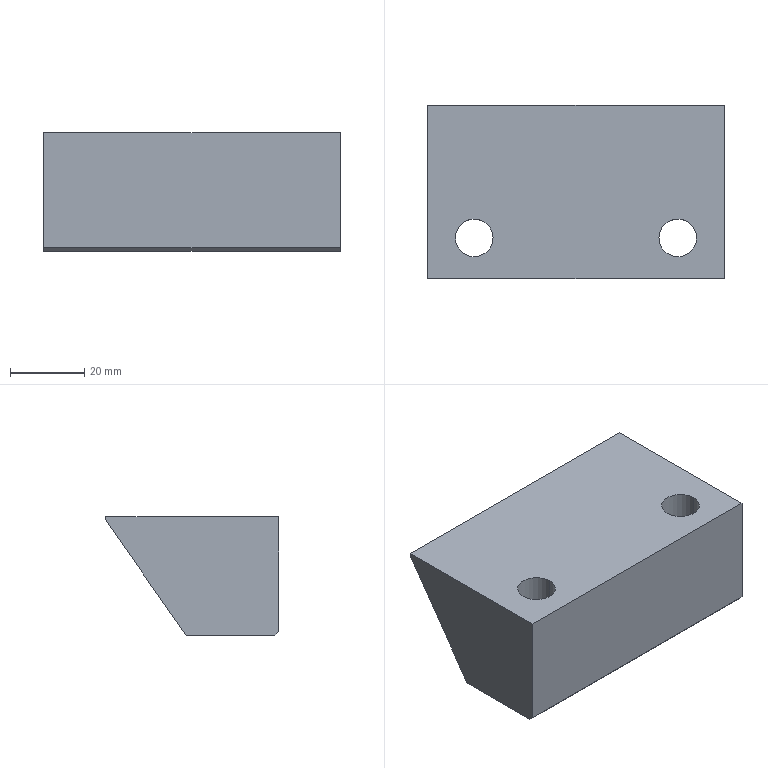Part | SolidWorks | features Chamfer 1, Extrusion 1, HoleWzd 1, MirrorPattern 1 | 1 solid | 16 faces | box 80 x 46.833 x 32 mm | volume 87358 mm3 | plane 8 | cone 4 | cylinder 4 | commonest cylinder face diameters 10.2 x4
STEP:
#1=CARTESIAN_POINT('',(72.6,11.,-31.075));
#2=VERTEX_POINT('',#1);
#3=CARTESIAN_POINT('',(62.4,11.,-31.075));
#4=VERTEX_POINT('',#3);
#5=CARTESIAN_POINT('',(67.5,11.,-31.075));
#6=DIRECTION('',(0.,0.,-1.));
#7=DIRECTION('',(-1.,0.,0.));
#8=AXIS2_PLACEMENT_3D('',#5,#6,#7);
#9=CIRCLE('',#8,5.1);
#10=EDGE_CURVE('',#2,#4,#9,.T.);
#11=ORIENTED_EDGE('',*,*,#10,.F.);
#12=CARTESIAN_POINT('',(73.525,11.,-32.));
#13=VERTEX_POINT('',#12);
#14=CARTESIAN_POINT('',(73.525,11.,-32.));
#15=DIRECTION('',(0.7071,0.,-0.7071));
#16=VECTOR('',#15,1000.);
#17=LINE('',#14,#16);
#18=EDGE_CURVE('',#2,#13,#17,.T.);
#19=ORIENTED_EDGE('',*,*,#18,.T.);
#20=CARTESIAN_POINT('',(61.475,11.,-32.));
#21=VERTEX_POINT('',#20);
#22=CARTESIAN_POINT('',(67.5,11.,-32.));
#23=DIRECTION('',(0.,0.,-1.));
#24=DIRECTION('',(-1.,0.,0.));
#25=AXIS2_PLACEMENT_3D('',#22,#23,#24);
#26=CIRCLE('',#25,6.025);
#27=EDGE_CURVE('',#13,#21,#26,.T.);
#28=ORIENTED_EDGE('',*,*,#27,.T.);
#29=CARTESIAN_POINT('',(61.475,11.,-32.));
#30=DIRECTION('',(-0.7071,0.,-0.7071));
#31=VECTOR('',#30,1000.);
#32=LINE('',#29,#31);
#33=EDGE_CURVE('',#4,#21,#32,.T.);
#34=ORIENTED_EDGE('',*,*,#33,.F.);
#35=EDGE_LOOP('',(#11,#19,#28,#34));
#36=FACE_OUTER_BOUND('',#35,.T.);
#37=CARTESIAN_POINT('',(67.5,11.,-32.));
#38=DIRECTION('',(0.,0.,-1.));
#39=DIRECTION('',(-1.,0.,0.));
#40=AXIS2_PLACEMENT_3D('',#37,#38,#39);
#41=CONICAL_SURFACE('',#40,6.025,0.7854);
#42=ADVANCED_FACE('',(#36),#41,.F.);
#43=CARTESIAN_POINT('',(72.6,11.,0.));
#44=VERTEX_POINT('',#43);
#45=CARTESIAN_POINT('',(62.4,11.,0.));
#46=VERTEX_POINT('',#45);
#47=CARTESIAN_POINT('',(67.5,11.,0.));
#48=DIRECTION('',(0.,0.,-1.));
#49=DIRECTION('',(0.,1.,0.));
#50=AXIS2_PLACEMENT_3D('',#47,#48,#49);
#51=CIRCLE('',#50,5.1);
#52=EDGE_CURVE('',#44,#46,#51,.T.);
#53=ORIENTED_EDGE('',*,*,#52,.F.);
#54=CARTESIAN_POINT('',(72.6,11.,-32.));
#55=DIRECTION('',(0.,0.,-1.));
#56=VECTOR('',#55,1000.);
#57=LINE('',#54,#56);
#58=EDGE_CURVE('',#44,#2,#57,.T.);
#59=ORIENTED_EDGE('',*,*,#58,.T.);
#60=ORIENTED_EDGE('',*,*,#10,.T.);
#61=CARTESIAN_POINT('',(62.4,11.,-32.));
#62=DIRECTION('',(0.,0.,-1.));
#63=VECTOR('',#62,1000.);
#64=LINE('',#61,#63);
#65=EDGE_CURVE('',#46,#4,#64,.T.);
#66=ORIENTED_EDGE('',*,*,#65,.F.);
#67=EDGE_LOOP('',(#53,#59,#60,#66));
#68=FACE_OUTER_BOUND('',#67,.T.);
#69=CARTESIAN_POINT('',(67.5,11.,-32.));
#70=DIRECTION('',(0.,0.,-1.));
#71=DIRECTION('',(-1.,0.,0.));
#72=AXIS2_PLACEMENT_3D('',#69,#70,#71);
#73=CYLINDRICAL_SURFACE('',#72,5.1);
#74=ADVANCED_FACE('',(#68),#73,.F.);
#75=CARTESIAN_POINT('',(17.6,11.,-31.075));
#76=VERTEX_POINT('',#75);
#77=CARTESIAN_POINT('',(7.4,11.,-31.075));
#78=VERTEX_POINT('',#77);
#79=CARTESIAN_POINT('',(12.5,11.,-31.075));
#80=DIRECTION('',(0.,0.,-1.));
#81=DIRECTION('',(-1.,0.,0.));
#82=AXIS2_PLACEMENT_3D('',#79,#80,#81);
#83=CIRCLE('',#82,5.1);
#84=EDGE_CURVE('',#76,#78,#83,.T.);
#85=ORIENTED_EDGE('',*,*,#84,.F.);
#86=CARTESIAN_POINT('',(18.525,11.,-32.));
#87=VERTEX_POINT('',#86);
#88=CARTESIAN_POINT('',(18.525,11.,-32.));
#89=DIRECTION('',(0.7071,0.,-0.7071));
#90=VECTOR('',#89,1000.);
#91=LINE('',#88,#90);
#92=EDGE_CURVE('',#76,#87,#91,.T.);
#93=ORIENTED_EDGE('',*,*,#92,.T.);
#94=CARTESIAN_POINT('',(6.475,11.,-32.));
#95=VERTEX_POINT('',#94);
#96=CARTESIAN_POINT('',(12.5,11.,-32.));
#97=DIRECTION('',(0.,0.,-1.));
#98=DIRECTION('',(-1.,0.,0.));
#99=AXIS2_PLACEMENT_3D('',#96,#97,#98);
#100=CIRCLE('',#99,6.025);
#101=EDGE_CURVE('',#87,#95,#100,.T.);
#102=ORIENTED_EDGE('',*,*,#101,.T.);
#103=CARTESIAN_POINT('',(6.475,11.,-32.));
#104=DIRECTION('',(-0.7071,0.,-0.7071));
#105=VECTOR('',#104,1000.);
#106=LINE('',#103,#105);
#107=EDGE_CURVE('',#78,#95,#106,.T.);
#108=ORIENTED_EDGE('',*,*,#107,.F.);
#109=EDGE_LOOP('',(#85,#93,#102,#108));
#110=FACE_OUTER_BOUND('',#109,.T.);
#111=CARTESIAN_POINT('',(12.5,11.,-32.));
#112=DIRECTION('',(0.,0.,-1.));
#113=DIRECTION('',(-1.,0.,0.));
#114=AXIS2_PLACEMENT_3D('',#111,#112,#113);
#115=CONICAL_SURFACE('',#114,6.025,0.7854);
#116=ADVANCED_FACE('',(#110),#115,.F.);
#117=CARTESIAN_POINT('',(17.6,11.,0.));
#118=VERTEX_POINT('',#117);
#119=CARTESIAN_POINT('',(7.4,11.,0.));
#120=VERTEX_POINT('',#119);
#121=CARTESIAN_POINT('',(12.5,11.,0.));
#122=DIRECTION('',(0.,0.,-1.));
#123=DIRECTION('',(0.,1.,0.));
#124=AXIS2_PLACEMENT_3D('',#121,#122,#123);
#125=CIRCLE('',#124,5.1);
#126=EDGE_CURVE('',#118,#120,#125,.T.);
#127=ORIENTED_EDGE('',*,*,#126,.F.);
#128=CARTESIAN_POINT('',(17.6,11.,-32.));
#129=DIRECTION('',(0.,0.,-1.));
#130=VECTOR('',#129,1000.);
#131=LINE('',#128,#130);
#132=EDGE_CURVE('',#118,#76,#131,.T.);
#133=ORIENTED_EDGE('',*,*,#132,.T.);
#134=ORIENTED_EDGE('',*,*,#84,.T.);
#135=CARTESIAN_POINT('',(7.4,11.,-32.));
#136=DIRECTION('',(0.,0.,-1.));
#137=VECTOR('',#136,1000.);
#138=LINE('',#135,#137);
#139=EDGE_CURVE('',#120,#78,#138,.T.);
#140=ORIENTED_EDGE('',*,*,#139,.F.);
#141=EDGE_LOOP('',(#127,#133,#134,#140));
#142=FACE_OUTER_BOUND('',#141,.T.);
#143=CARTESIAN_POINT('',(12.5,11.,-32.));
#144=DIRECTION('',(0.,0.,-1.));
#145=DIRECTION('',(-1.,0.,0.));
#146=AXIS2_PLACEMENT_3D('',#143,#144,#145);
#147=CYLINDRICAL_SURFACE('',#146,5.1);
#148=ADVANCED_FACE('',(#142),#147,.F.);
#149=CARTESIAN_POINT('',(0.,0.,0.));
#150=VERTEX_POINT('',#149);
#151=CARTESIAN_POINT('',(0.,0.,-31.));
#152=VERTEX_POINT('',#151);
#153=CARTESIAN_POINT('',(0.,0.,-32.));
#154=DIRECTION('',(0.,0.,-1.));
#155=VECTOR('',#154,1000.);
#156=LINE('',#153,#155);
#157=EDGE_CURVE('',#150,#152,#156,.T.);
#158=ORIENTED_EDGE('',*,*,#157,.T.);
#159=CARTESIAN_POINT('',(80.,0.,-31.));
#160=VERTEX_POINT('',#159);
#161=CARTESIAN_POINT('',(80.,0.,-31.));
#162=DIRECTION('',(1.,0.,0.));
#163=VECTOR('',#162,1000.);
#164=LINE('',#161,#163);
#165=EDGE_CURVE('',#152,#160,#164,.T.);
#166=ORIENTED_EDGE('',*,*,#165,.T.);
#167=CARTESIAN_POINT('',(80.,0.,0.));
#168=VERTEX_POINT('',#167);
#169=CARTESIAN_POINT('',(80.,0.,-32.));
#170=DIRECTION('',(0.,0.,-1.));
#171=VECTOR('',#170,1000.);
#172=LINE('',#169,#171);
#173=EDGE_CURVE('',#168,#160,#172,.T.);
#174=ORIENTED_EDGE('',*,*,#173,.F.);
#175=CARTESIAN_POINT('',(80.,0.,0.));
#176=DIRECTION('',(-1.,0.,0.));
#177=VECTOR('',#176,1000.);
#178=LINE('',#175,#177);
#179=EDGE_CURVE('',#168,#150,#178,.T.);
#180=ORIENTED_EDGE('',*,*,#179,.T.);
#181=EDGE_LOOP('',(#158,#166,#174,#180));
#182=FACE_OUTER_BOUND('',#181,.T.);
#183=CARTESIAN_POINT('',(80.,0.,-32.));
#184=DIRECTION('',(0.,1.,0.));
#185=DIRECTION('',(0.,0.,1.));
#186=AXIS2_PLACEMENT_3D('',#183,#184,#185);
#187=PLANE('',#186);
#188=ADVANCED_FACE('',(#182),#187,.F.);
#189=CARTESIAN_POINT('',(67.5,11.,-32.));
#190=DIRECTION('',(0.,0.,-1.));
#191=DIRECTION('',(-1.,0.,0.));
#192=AXIS2_PLACEMENT_3D('',#189,#190,#191);
#193=CIRCLE('',#192,6.025);
#194=EDGE_CURVE('',#21,#13,#193,.T.);
#195=ORIENTED_EDGE('',*,*,#194,.F.);
#196=ORIENTED_EDGE('',*,*,#27,.F.);
#197=EDGE_LOOP('',(#195,#196));
#198=FACE_BOUND('',#197,.T.);
#199=CARTESIAN_POINT('',(12.5,11.,-32.));
#200=DIRECTION('',(0.,0.,-1.));
#201=DIRECTION('',(-1.,0.,0.));
#202=AXIS2_PLACEMENT_3D('',#199,#200,#201);
#203=CIRCLE('',#202,6.025);
#204=EDGE_CURVE('',#95,#87,#203,.T.);
#205=ORIENTED_EDGE('',*,*,#204,.F.);
#206=ORIENTED_EDGE('',*,*,#101,.F.);
#207=EDGE_LOOP('',(#205,#206));
#208=FACE_BOUND('',#207,.T.);
#209=CARTESIAN_POINT('',(80.,1.,-32.));
#210=VERTEX_POINT('',#209);
#211=CARTESIAN_POINT('',(80.,25.,-32.));
#212=VERTEX_POINT('',#211);
#213=CARTESIAN_POINT('',(80.,25.,-32.));
#214=DIRECTION('',(0.,1.,0.));
#215=VECTOR('',#214,1000.);
#216=LINE('',#213,#215);
#217=EDGE_CURVE('',#210,#212,#216,.T.);
#218=ORIENTED_EDGE('',*,*,#217,.F.);
#219=CARTESIAN_POINT('',(0.,1.,-32.));
#220=VERTEX_POINT('',#219);
#221=CARTESIAN_POINT('',(80.,1.,-32.));
#222=DIRECTION('',(-1.,0.,0.));
#223=VECTOR('',#222,1000.);
#224=LINE('',#221,#223);
#225=EDGE_CURVE('',#210,#220,#224,.T.);
#226=ORIENTED_EDGE('',*,*,#225,.T.);
#227=CARTESIAN_POINT('',(0.,25.,-32.));
#228=VERTEX_POINT('',#227);
#229=CARTESIAN_POINT('',(0.,25.,-32.));
#230=DIRECTION('',(0.,1.,0.));
#231=VECTOR('',#230,1000.);
#232=LINE('',#229,#231);
#233=EDGE_CURVE('',#220,#228,#232,.T.);
#234=ORIENTED_EDGE('',*,*,#233,.T.);
#235=CARTESIAN_POINT('',(80.,25.,-32.));
#236=DIRECTION('',(-1.,0.,0.));
#237=VECTOR('',#236,1000.);
#238=LINE('',#235,#237);
#239=EDGE_CURVE('',#212,#228,#238,.T.);
#240=ORIENTED_EDGE('',*,*,#239,.F.);
#241=EDGE_LOOP('',(#218,#226,#234,#240));
#242=FACE_OUTER_BOUND('',#241,.T.);
#243=CARTESIAN_POINT('',(80.,25.,-32.));
#244=DIRECTION('',(0.,0.,1.));
#245=DIRECTION('',(1.,0.,0.));
#246=AXIS2_PLACEMENT_3D('',#243,#244,#245);
#247=PLANE('',#246);
#248=ADVANCED_FACE('',(#198,#208,#242),#247,.F.);
#249=CARTESIAN_POINT('',(0.,46.833,-0.8192));
#250=VERTEX_POINT('',#249);
#251=CARTESIAN_POINT('',(0.,47.407,0.));
#252=DIRECTION('',(0.,0.5736,0.8192));
#253=VECTOR('',#252,1000.);
#254=LINE('',#251,#253);
#255=EDGE_CURVE('',#228,#250,#254,.T.);
#256=ORIENTED_EDGE('',*,*,#255,.T.);
#257=CARTESIAN_POINT('',(80.,46.833,-0.8192));
#258=VERTEX_POINT('',#257);
#259=CARTESIAN_POINT('',(80.,46.833,-0.8192));
#260=DIRECTION('',(1.,0.,0.));
#261=VECTOR('',#260,1000.);
#262=LINE('',#259,#261);
#263=EDGE_CURVE('',#250,#258,#262,.T.);
#264=ORIENTED_EDGE('',*,*,#263,.T.);
#265=CARTESIAN_POINT('',(80.,47.407,0.));
#266=DIRECTION('',(0.,0.5736,0.8192));
#267=VECTOR('',#266,1000.);
#268=LINE('',#265,#267);
#269=EDGE_CURVE('',#212,#258,#268,.T.);
#270=ORIENTED_EDGE('',*,*,#269,.F.);
#271=ORIENTED_EDGE('',*,*,#239,.T.);
#272=EDGE_LOOP('',(#256,#264,#270,#271));
#273=FACE_OUTER_BOUND('',#272,.T.);
#274=CARTESIAN_POINT('',(80.,47.407,0.));
#275=DIRECTION('',(0.,-0.8192,0.5736));
#276=DIRECTION('',(0.,-0.5736,-0.8192));
#277=AXIS2_PLACEMENT_3D('',#274,#275,#276);
#278=PLANE('',#277);
#279=ADVANCED_FACE('',(#273),#278,.F.);
#280=CARTESIAN_POINT('',(67.5,11.,0.));
#281=DIRECTION('',(0.,0.,-1.));
#282=DIRECTION('',(0.,1.,0.));
#283=AXIS2_PLACEMENT_3D('',#280,#281,#282);
#284=CIRCLE('',#283,5.1);
#285=EDGE_CURVE('',#46,#44,#284,.T.);
#286=ORIENTED_EDGE('',*,*,#285,.T.);
#287=ORIENTED_EDGE('',*,*,#52,.T.);
#288=EDGE_LOOP('',(#286,#287));
#289=FACE_BOUND('',#288,.T.);
#290=CARTESIAN_POINT('',(12.5,11.,0.));
#291=DIRECTION('',(0.,0.,-1.));
#292=DIRECTION('',(0.,1.,0.));
#293=AXIS2_PLACEMENT_3D('',#290,#291,#292);
#294=CIRCLE('',#293,5.1);
#295=EDGE_CURVE('',#120,#118,#294,.T.);
#296=ORIENTED_EDGE('',*,*,#295,.T.);
#297=ORIENTED_EDGE('',*,*,#126,.T.);
#298=EDGE_LOOP('',(#296,#297));
#299=FACE_BOUND('',#298,.T.);
#300=CARTESIAN_POINT('',(80.,46.689,0.));
#301=VERTEX_POINT('',#300);
#302=CARTESIAN_POINT('',(80.,0.,0.));
#303=DIRECTION('',(0.,-1.,0.));
#304=VECTOR('',#303,1000.);
#305=LINE('',#302,#304);
#306=EDGE_CURVE('',#301,#168,#305,.T.);
#307=ORIENTED_EDGE('',*,*,#306,.F.);
#308=CARTESIAN_POINT('',(0.,46.689,0.));
#309=VERTEX_POINT('',#308);
#310=CARTESIAN_POINT('',(80.,46.689,0.));
#311=DIRECTION('',(-1.,0.,0.));
#312=VECTOR('',#311,1000.);
#313=LINE('',#310,#312);
#314=EDGE_CURVE('',#301,#309,#313,.T.);
#315=ORIENTED_EDGE('',*,*,#314,.T.);
#316=CARTESIAN_POINT('',(0.,0.,0.));
#317=DIRECTION('',(0.,-1.,0.));
#318=VECTOR('',#317,1000.);
#319=LINE('',#316,#318);
#320=EDGE_CURVE('',#309,#150,#319,.T.);
#321=ORIENTED_EDGE('',*,*,#320,.T.);
#322=ORIENTED_EDGE('',*,*,#179,.F.);
#323=EDGE_LOOP('',(#307,#315,#321,#322));
#324=FACE_OUTER_BOUND('',#323,.T.);
#325=CARTESIAN_POINT('',(80.,0.,0.));
#326=DIRECTION('',(0.,0.,-1.));
#327=DIRECTION('',(0.,1.,0.));
#328=AXIS2_PLACEMENT_3D('',#325,#326,#327);
#329=PLANE('',#328);
#330=ADVANCED_FACE('',(#289,#299,#324),#329,.F.);
#331=ORIENTED_EDGE('',*,*,#173,.T.);
#332=CARTESIAN_POINT('',(80.,1.,-32.));
#333=DIRECTION('',(0.,0.7071,-0.7071));
#334=VECTOR('',#333,1000.);
#335=LINE('',#332,#334);
#336=EDGE_CURVE('',#160,#210,#335,.T.);
#337=ORIENTED_EDGE('',*,*,#336,.T.);
#338=ORIENTED_EDGE('',*,*,#217,.T.);
#339=ORIENTED_EDGE('',*,*,#269,.T.);
#340=CARTESIAN_POINT('',(80.,46.689,0.));
#341=DIRECTION('',(0.,-0.1736,0.9848));
#342=VECTOR('',#341,1000.);
#343=LINE('',#340,#342);
#344=EDGE_CURVE('',#258,#301,#343,.T.);
#345=ORIENTED_EDGE('',*,*,#344,.T.);
#346=ORIENTED_EDGE('',*,*,#306,.T.);
#347=EDGE_LOOP('',(#331,#337,#338,#339,#345,#346));
#348=FACE_OUTER_BOUND('',#347,.T.);
#349=CARTESIAN_POINT('',(80.,0.,0.));
#350=DIRECTION('',(-1.,0.,0.));
#351=DIRECTION('',(0.,0.,1.));
#352=AXIS2_PLACEMENT_3D('',#349,#350,#351);
#353=PLANE('',#352);
#354=ADVANCED_FACE('',(#348),#353,.F.);
#355=ORIENTED_EDGE('',*,*,#233,.F.);
#356=CARTESIAN_POINT('',(0.,-15.5,-15.5));
#357=DIRECTION('',(0.,-0.7071,0.7071));
#358=VECTOR('',#357,1000.);
#359=LINE('',#356,#358);
#360=EDGE_CURVE('',#220,#152,#359,.T.);
#361=ORIENTED_EDGE('',*,*,#360,.T.);
#362=ORIENTED_EDGE('',*,*,#157,.F.);
#363=ORIENTED_EDGE('',*,*,#320,.F.);
#364=CARTESIAN_POINT('',(0.,45.281,7.984));
#365=DIRECTION('',(0.,0.1736,-0.9848));
#366=VECTOR('',#365,1000.);
#367=LINE('',#364,#366);
#368=EDGE_CURVE('',#309,#250,#367,.T.);
#369=ORIENTED_EDGE('',*,*,#368,.T.);
#370=ORIENTED_EDGE('',*,*,#255,.F.);
#371=EDGE_LOOP('',(#355,#361,#362,#363,#369,#370));
#372=FACE_OUTER_BOUND('',#371,.T.);
#373=CARTESIAN_POINT('',(0.,0.,0.));
#374=DIRECTION('',(-1.,0.,0.));
#375=DIRECTION('',(0.,0.,1.));
#376=AXIS2_PLACEMENT_3D('',#373,#374,#375);
#377=PLANE('',#376);
#378=ADVANCED_FACE('',(#372),#377,.T.);
#379=ORIENTED_EDGE('',*,*,#132,.F.);
#380=ORIENTED_EDGE('',*,*,#295,.F.);
#381=ORIENTED_EDGE('',*,*,#139,.T.);
#382=CARTESIAN_POINT('',(12.5,11.,-31.075));
#383=DIRECTION('',(0.,0.,-1.));
#384=DIRECTION('',(-1.,0.,0.));
#385=AXIS2_PLACEMENT_3D('',#382,#383,#384);
#386=CIRCLE('',#385,5.1);
#387=EDGE_CURVE('',#78,#76,#386,.T.);
#388=ORIENTED_EDGE('',*,*,#387,.T.);
#389=EDGE_LOOP('',(#379,#380,#381,#388));
#390=FACE_OUTER_BOUND('',#389,.T.);
#391=CARTESIAN_POINT('',(12.5,11.,-32.));
#392=DIRECTION('',(0.,0.,-1.));
#393=DIRECTION('',(-1.,0.,0.));
#394=AXIS2_PLACEMENT_3D('',#391,#392,#393);
#395=CYLINDRICAL_SURFACE('',#394,5.1);
#396=ADVANCED_FACE('',(#390),#395,.F.);
#397=ORIENTED_EDGE('',*,*,#92,.F.);
#398=ORIENTED_EDGE('',*,*,#387,.F.);
#399=ORIENTED_EDGE('',*,*,#107,.T.);
#400=ORIENTED_EDGE('',*,*,#204,.T.);
#401=EDGE_LOOP('',(#397,#398,#399,#400));
#402=FACE_OUTER_BOUND('',#401,.T.);
#403=CARTESIAN_POINT('',(12.5,11.,-32.));
#404=DIRECTION('',(0.,0.,-1.));
#405=DIRECTION('',(-1.,0.,0.));
#406=AXIS2_PLACEMENT_3D('',#403,#404,#405);
#407=CONICAL_SURFACE('',#406,6.025,0.7854);
#408=ADVANCED_FACE('',(#402),#407,.F.);
#409=ORIENTED_EDGE('',*,*,#58,.F.);
#410=ORIENTED_EDGE('',*,*,#285,.F.);
#411=ORIENTED_EDGE('',*,*,#65,.T.);
#412=CARTESIAN_POINT('',(67.5,11.,-31.075));
#413=DIRECTION('',(0.,0.,-1.));
#414=DIRECTION('',(-1.,0.,0.));
#415=AXIS2_PLACEMENT_3D('',#412,#413,#414);
#416=CIRCLE('',#415,5.1);
#417=EDGE_CURVE('',#4,#2,#416,.T.);
#418=ORIENTED_EDGE('',*,*,#417,.T.);
#419=EDGE_LOOP('',(#409,#410,#411,#418));
#420=FACE_OUTER_BOUND('',#419,.T.);
#421=CARTESIAN_POINT('',(67.5,11.,-32.));
#422=DIRECTION('',(0.,0.,-1.));
#423=DIRECTION('',(-1.,0.,0.));
#424=AXIS2_PLACEMENT_3D('',#421,#422,#423);
#425=CYLINDRICAL_SURFACE('',#424,5.1);
#426=ADVANCED_FACE('',(#420),#425,.F.);
#427=ORIENTED_EDGE('',*,*,#18,.F.);
#428=ORIENTED_EDGE('',*,*,#417,.F.);
#429=ORIENTED_EDGE('',*,*,#33,.T.);
#430=ORIENTED_EDGE('',*,*,#194,.T.);
#431=EDGE_LOOP('',(#427,#428,#429,#430));
#432=FACE_OUTER_BOUND('',#431,.T.);
#433=CARTESIAN_POINT('',(67.5,11.,-32.));
#434=DIRECTION('',(0.,0.,-1.));
#435=DIRECTION('',(-1.,0.,0.));
#436=AXIS2_PLACEMENT_3D('',#433,#434,#435);
#437=CONICAL_SURFACE('',#436,6.025,0.7854);
#438=ADVANCED_FACE('',(#432),#437,.F.);
#439=ORIENTED_EDGE('',*,*,#336,.F.);
#440=ORIENTED_EDGE('',*,*,#165,.F.);
#441=ORIENTED_EDGE('',*,*,#360,.F.);
#442=ORIENTED_EDGE('',*,*,#225,.F.);
#443=EDGE_LOOP('',(#439,#440,#441,#442));
#444=FACE_OUTER_BOUND('',#443,.T.);
#445=CARTESIAN_POINT('',(80.,1.,-32.));
#446=DIRECTION('',(0.,0.7071,0.7071));
#447=DIRECTION('',(-1.,0.,0.));
#448=AXIS2_PLACEMENT_3D('',#445,#446,#447);
#449=PLANE('',#448);
#450=ADVANCED_FACE('',(#444),#449,.F.);
#451=ORIENTED_EDGE('',*,*,#344,.F.);
#452=ORIENTED_EDGE('',*,*,#263,.F.);
#453=ORIENTED_EDGE('',*,*,#368,.F.);
#454=ORIENTED_EDGE('',*,*,#314,.F.);
#455=EDGE_LOOP('',(#451,#452,#453,#454));
#456=FACE_OUTER_BOUND('',#455,.T.);
#457=CARTESIAN_POINT('',(80.,46.689,0.));
#458=DIRECTION('',(0.,-0.9848,-0.1736));
#459=DIRECTION('',(-1.,0.,0.));
#460=AXIS2_PLACEMENT_3D('',#457,#458,#459);
#461=PLANE('',#460);
#462=ADVANCED_FACE('',(#456),#461,.F.);
#463=CLOSED_SHELL('',(#42,#74,#116,#148,#188,#248,#279,#330,#354,#378,#396,#408,#426,#438,#450,#462));
#464=MANIFOLD_SOLID_BREP('',#463);
#465=CARTESIAN_POINT('',(0.,0.,0.));
#466=DIRECTION('',(0.,0.,1.));
#467=DIRECTION('',(1.,0.,0.));
#468=AXIS2_PLACEMENT_3D('',#465,#466,#467);
#469=(LENGTH_UNIT()NAMED_UNIT(*)SI_UNIT(.MILLI.,.METRE.));
#470=UNCERTAINTY_MEASURE_WITH_UNIT(LENGTH_MEASURE(0.00001),#469,'','');
#471=(NAMED_UNIT(*)PLANE_ANGLE_UNIT()SI_UNIT($,.RADIAN.));
#472=(NAMED_UNIT(*)SI_UNIT($,.STERADIAN.)SOLID_ANGLE_UNIT());
#473=(GEOMETRIC_REPRESENTATION_CONTEXT(3)GLOBAL_UNCERTAINTY_ASSIGNED_CONTEXT((#470))GLOBAL_UNIT_ASSIGNED_CONTEXT((#469,#471,#472))REPRESENTATION_CONTEXT('',''));
#474=ADVANCED_BREP_SHAPE_REPRESENTATION('',(#464,#468),#473);